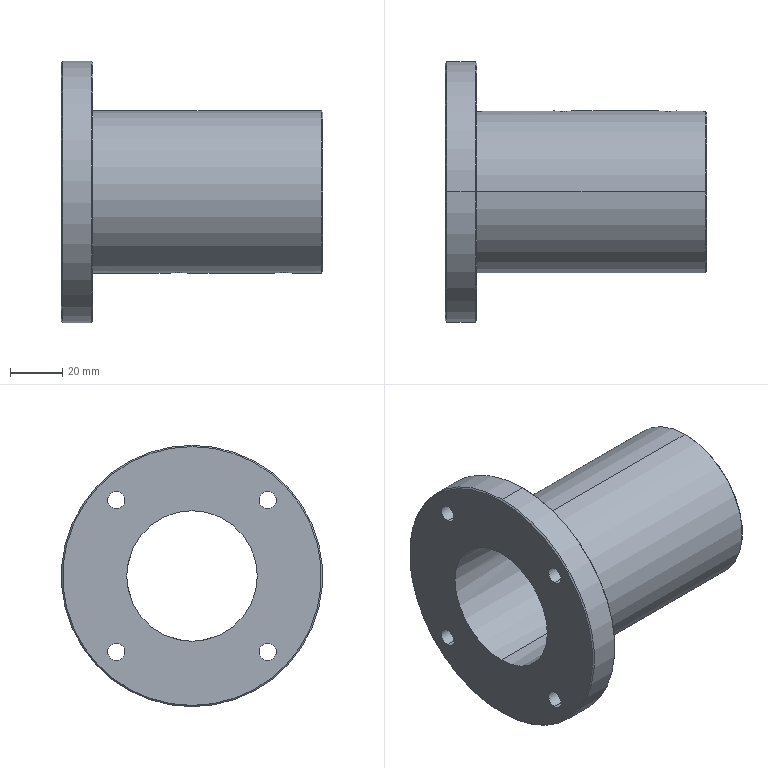Part | STEP file | TJ-DHQM-003-002_STHRBK30 | 1 solid | 33 faces | box 100 x 100 x 100 mm | volume 160939 mm3 | cylinder 22 | cone 8 | plane 3 | commonest cylinder face diameters 6.6 x8 6.8 x8 50 x2 62 x2 100 x2